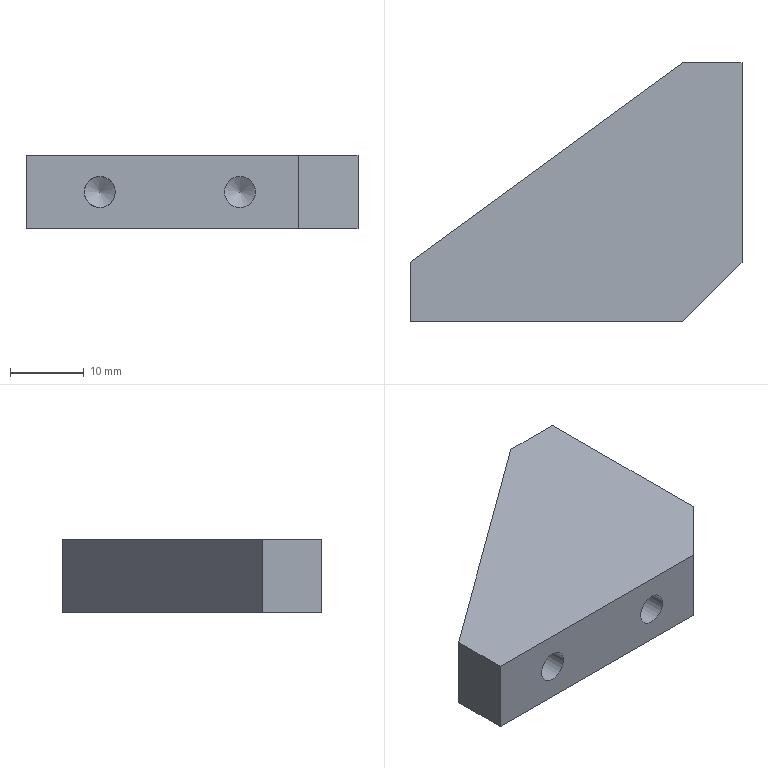Part | NX | features BREP 1 | 1 solid | 14 faces | box 45 x 35 x 10 mm | volume 9902 mm3 | plane 8 | cylinder 3 | cone 3 | commonest cylinder face diameters 4.2 x3
STEP:
#1=CARTESIAN_POINT('',(-45.,8.,10.));
#2=VERTEX_POINT('',#1);
#3=CARTESIAN_POINT('',(-45.,0.,10.));
#4=VERTEX_POINT('',#3);
#5=CARTESIAN_POINT('',(-45.,0.,10.));
#6=DIRECTION('',(0.,-1.,0.));
#7=VECTOR('',#6,1000.);
#8=LINE('',#5,#7);
#9=EDGE_CURVE('',#2,#4,#8,.T.);
#10=ORIENTED_EDGE('',*,*,#9,.T.);
#11=CARTESIAN_POINT('',(-8.,0.,10.));
#12=VERTEX_POINT('',#11);
#13=CARTESIAN_POINT('',(0.,0.,10.));
#14=DIRECTION('',(1.,0.,0.));
#15=VECTOR('',#14,1000.);
#16=LINE('',#13,#15);
#17=EDGE_CURVE('',#4,#12,#16,.T.);
#18=ORIENTED_EDGE('',*,*,#17,.T.);
#19=CARTESIAN_POINT('',(0.,8.,10.));
#20=VERTEX_POINT('',#19);
#21=CARTESIAN_POINT('',(-8.,0.,10.));
#22=DIRECTION('',(0.7071,0.7071,0.));
#23=VECTOR('',#22,1000.);
#24=LINE('',#21,#23);
#25=EDGE_CURVE('',#12,#20,#24,.T.);
#26=ORIENTED_EDGE('',*,*,#25,.T.);
#27=CARTESIAN_POINT('',(0.,35.,10.));
#28=VERTEX_POINT('',#27);
#29=CARTESIAN_POINT('',(0.,0.,10.));
#30=DIRECTION('',(0.,1.,0.));
#31=VECTOR('',#30,1000.);
#32=LINE('',#29,#31);
#33=EDGE_CURVE('',#20,#28,#32,.T.);
#34=ORIENTED_EDGE('',*,*,#33,.T.);
#35=CARTESIAN_POINT('',(-8.,35.,10.));
#36=VERTEX_POINT('',#35);
#37=CARTESIAN_POINT('',(0.,35.,10.));
#38=DIRECTION('',(-1.,0.,0.));
#39=VECTOR('',#38,1000.);
#40=LINE('',#37,#39);
#41=EDGE_CURVE('',#28,#36,#40,.T.);
#42=ORIENTED_EDGE('',*,*,#41,.T.);
#43=CARTESIAN_POINT('',(-8.,35.,10.));
#44=DIRECTION('',(-0.8078,-0.5895,0.));
#45=VECTOR('',#44,1000.);
#46=LINE('',#43,#45);
#47=EDGE_CURVE('',#36,#2,#46,.T.);
#48=ORIENTED_EDGE('',*,*,#47,.T.);
#49=EDGE_LOOP('',(#10,#18,#26,#34,#42,#48));
#50=FACE_BOUND('',#49,.T.);
#51=CARTESIAN_POINT('',(0.,0.,10.));
#52=DIRECTION('',(0.,0.,1.));
#53=DIRECTION('',(-1.,0.,0.));
#54=AXIS2_PLACEMENT_3D('',#51,#52,#53);
#55=PLANE('',#54);
#56=ADVANCED_FACE('',(#50),#55,.T.);
#57=CARTESIAN_POINT('',(-8.,0.,0.));
#58=VERTEX_POINT('',#57);
#59=CARTESIAN_POINT('',(-8.,0.,10.));
#60=DIRECTION('',(0.,0.,-1.));
#61=VECTOR('',#60,1000.);
#62=LINE('',#59,#61);
#63=EDGE_CURVE('',#12,#58,#62,.T.);
#64=ORIENTED_EDGE('',*,*,#63,.F.);
#65=ORIENTED_EDGE('',*,*,#17,.F.);
#66=CARTESIAN_POINT('',(-45.,0.,0.));
#67=VERTEX_POINT('',#66);
#68=CARTESIAN_POINT('',(-45.,0.,10.));
#69=DIRECTION('',(0.,0.,1.));
#70=VECTOR('',#69,1000.);
#71=LINE('',#68,#70);
#72=EDGE_CURVE('',#67,#4,#71,.T.);
#73=ORIENTED_EDGE('',*,*,#72,.F.);
#74=CARTESIAN_POINT('',(-45.,0.,0.));
#75=DIRECTION('',(-1.,0.,0.));
#76=VECTOR('',#75,1000.);
#77=LINE('',#74,#76);
#78=EDGE_CURVE('',#58,#67,#77,.T.);
#79=ORIENTED_EDGE('',*,*,#78,.F.);
#80=EDGE_LOOP('',(#64,#65,#73,#79));
#81=FACE_BOUND('',#80,.T.);
#82=CARTESIAN_POINT('',(-16.,0.,2.9));
#83=VERTEX_POINT('',#82);
#84=CARTESIAN_POINT('',(-16.,0.,5.));
#85=DIRECTION('',(0.,-1.,0.));
#86=DIRECTION('',(0.,0.,-1.));
#87=AXIS2_PLACEMENT_3D('',#84,#85,#86);
#88=CIRCLE('',#87,2.1);
#89=EDGE_CURVE('',#83,#83,#88,.T.);
#90=ORIENTED_EDGE('',*,*,#89,.F.);
#91=EDGE_LOOP('',(#90));
#92=FACE_BOUND('',#91,.T.);
#93=CARTESIAN_POINT('',(-35.,0.,2.9));
#94=VERTEX_POINT('',#93);
#95=CARTESIAN_POINT('',(-35.,0.,5.));
#96=DIRECTION('',(0.,-1.,0.));
#97=DIRECTION('',(0.,0.,-1.));
#98=AXIS2_PLACEMENT_3D('',#95,#96,#97);
#99=CIRCLE('',#98,2.1);
#100=EDGE_CURVE('',#94,#94,#99,.T.);
#101=ORIENTED_EDGE('',*,*,#100,.F.);
#102=EDGE_LOOP('',(#101));
#103=FACE_BOUND('',#102,.T.);
#104=CARTESIAN_POINT('',(-45.,0.,10.));
#105=DIRECTION('',(0.,1.,0.));
#106=DIRECTION('',(0.,0.,-1.));
#107=AXIS2_PLACEMENT_3D('',#104,#105,#106);
#108=PLANE('',#107);
#109=ADVANCED_FACE('',(#81,#92,#103),#108,.F.);
#110=ORIENTED_EDGE('',*,*,#72,.T.);
#111=ORIENTED_EDGE('',*,*,#9,.F.);
#112=CARTESIAN_POINT('',(-45.,8.,0.));
#113=VERTEX_POINT('',#112);
#114=CARTESIAN_POINT('',(-45.,8.,10.));
#115=DIRECTION('',(0.,0.,1.));
#116=VECTOR('',#115,1000.);
#117=LINE('',#114,#116);
#118=EDGE_CURVE('',#113,#2,#117,.T.);
#119=ORIENTED_EDGE('',*,*,#118,.F.);
#120=CARTESIAN_POINT('',(-45.,8.,0.));
#121=DIRECTION('',(0.,1.,0.));
#122=VECTOR('',#121,1000.);
#123=LINE('',#120,#122);
#124=EDGE_CURVE('',#67,#113,#123,.T.);
#125=ORIENTED_EDGE('',*,*,#124,.F.);
#126=EDGE_LOOP('',(#110,#111,#119,#125));
#127=FACE_BOUND('',#126,.T.);
#128=CARTESIAN_POINT('',(-45.,8.,10.));
#129=DIRECTION('',(1.,0.,0.));
#130=DIRECTION('',(0.,0.,1.));
#131=AXIS2_PLACEMENT_3D('',#128,#129,#130);
#132=PLANE('',#131);
#133=ADVANCED_FACE('',(#127),#132,.F.);
#134=ORIENTED_EDGE('',*,*,#118,.T.);
#135=ORIENTED_EDGE('',*,*,#47,.F.);
#136=CARTESIAN_POINT('',(-8.,35.,0.));
#137=VERTEX_POINT('',#136);
#138=CARTESIAN_POINT('',(-8.,35.,10.));
#139=DIRECTION('',(0.,0.,1.));
#140=VECTOR('',#139,1000.);
#141=LINE('',#138,#140);
#142=EDGE_CURVE('',#137,#36,#141,.T.);
#143=ORIENTED_EDGE('',*,*,#142,.F.);
#144=CARTESIAN_POINT('',(-8.,35.,0.));
#145=DIRECTION('',(0.8078,0.5895,0.));
#146=VECTOR('',#145,1000.);
#147=LINE('',#144,#146);
#148=EDGE_CURVE('',#113,#137,#147,.T.);
#149=ORIENTED_EDGE('',*,*,#148,.F.);
#150=EDGE_LOOP('',(#134,#135,#143,#149));
#151=FACE_BOUND('',#150,.T.);
#152=CARTESIAN_POINT('',(-8.,35.,10.));
#153=DIRECTION('',(0.5895,-0.8078,0.));
#154=DIRECTION('',(-0.8078,-0.5895,0.));
#155=AXIS2_PLACEMENT_3D('',#152,#153,#154);
#156=PLANE('',#155);
#157=ADVANCED_FACE('',(#151),#156,.F.);
#158=ORIENTED_EDGE('',*,*,#142,.T.);
#159=ORIENTED_EDGE('',*,*,#41,.F.);
#160=CARTESIAN_POINT('',(0.,35.,0.));
#161=VERTEX_POINT('',#160);
#162=CARTESIAN_POINT('',(0.,35.,10.));
#163=DIRECTION('',(0.,0.,1.));
#164=VECTOR('',#163,1000.);
#165=LINE('',#162,#164);
#166=EDGE_CURVE('',#161,#28,#165,.T.);
#167=ORIENTED_EDGE('',*,*,#166,.F.);
#168=CARTESIAN_POINT('',(0.,35.,0.));
#169=DIRECTION('',(1.,0.,0.));
#170=VECTOR('',#169,1000.);
#171=LINE('',#168,#170);
#172=EDGE_CURVE('',#137,#161,#171,.T.);
#173=ORIENTED_EDGE('',*,*,#172,.F.);
#174=EDGE_LOOP('',(#158,#159,#167,#173));
#175=FACE_BOUND('',#174,.T.);
#176=CARTESIAN_POINT('',(0.,35.,10.));
#177=DIRECTION('',(0.,-1.,0.));
#178=DIRECTION('',(0.,0.,1.));
#179=AXIS2_PLACEMENT_3D('',#176,#177,#178);
#180=PLANE('',#179);
#181=ADVANCED_FACE('',(#175),#180,.F.);
#182=ORIENTED_EDGE('',*,*,#166,.T.);
#183=ORIENTED_EDGE('',*,*,#33,.F.);
#184=CARTESIAN_POINT('',(0.,8.,0.));
#185=VERTEX_POINT('',#184);
#186=CARTESIAN_POINT('',(0.,8.,10.));
#187=DIRECTION('',(0.,0.,1.));
#188=VECTOR('',#187,1000.);
#189=LINE('',#186,#188);
#190=EDGE_CURVE('',#185,#20,#189,.T.);
#191=ORIENTED_EDGE('',*,*,#190,.F.);
#192=CARTESIAN_POINT('',(0.,8.,0.));
#193=DIRECTION('',(0.,-1.,0.));
#194=VECTOR('',#193,1000.);
#195=LINE('',#192,#194);
#196=EDGE_CURVE('',#161,#185,#195,.T.);
#197=ORIENTED_EDGE('',*,*,#196,.F.);
#198=EDGE_LOOP('',(#182,#183,#191,#197));
#199=FACE_BOUND('',#198,.T.);
#200=CARTESIAN_POINT('',(0.,25.,2.9));
#201=VERTEX_POINT('',#200);
#202=CARTESIAN_POINT('',(0.,25.,5.));
#203=DIRECTION('',(1.,0.,0.));
#204=DIRECTION('',(0.,0.,-1.));
#205=AXIS2_PLACEMENT_3D('',#202,#203,#204);
#206=CIRCLE('',#205,2.1);
#207=EDGE_CURVE('',#201,#201,#206,.T.);
#208=ORIENTED_EDGE('',*,*,#207,.F.);
#209=EDGE_LOOP('',(#208));
#210=FACE_BOUND('',#209,.T.);
#211=CARTESIAN_POINT('',(0.,8.,10.));
#212=DIRECTION('',(-1.,0.,0.));
#213=DIRECTION('',(0.,0.,-1.));
#214=AXIS2_PLACEMENT_3D('',#211,#212,#213);
#215=PLANE('',#214);
#216=ADVANCED_FACE('',(#199,#210),#215,.F.);
#217=ORIENTED_EDGE('',*,*,#190,.T.);
#218=ORIENTED_EDGE('',*,*,#25,.F.);
#219=ORIENTED_EDGE('',*,*,#63,.T.);
#220=CARTESIAN_POINT('',(-8.,0.,0.));
#221=DIRECTION('',(-0.7071,-0.7071,0.));
#222=VECTOR('',#221,1000.);
#223=LINE('',#220,#222);
#224=EDGE_CURVE('',#185,#58,#223,.T.);
#225=ORIENTED_EDGE('',*,*,#224,.F.);
#226=EDGE_LOOP('',(#217,#218,#219,#225));
#227=FACE_BOUND('',#226,.T.);
#228=CARTESIAN_POINT('',(-8.,0.,10.));
#229=DIRECTION('',(-0.7071,0.7071,0.));
#230=DIRECTION('',(0.7071,0.7071,0.));
#231=AXIS2_PLACEMENT_3D('',#228,#229,#230);
#232=PLANE('',#231);
#233=ADVANCED_FACE('',(#227),#232,.F.);
#234=ORIENTED_EDGE('',*,*,#78,.T.);
#235=ORIENTED_EDGE('',*,*,#124,.T.);
#236=ORIENTED_EDGE('',*,*,#148,.T.);
#237=ORIENTED_EDGE('',*,*,#172,.T.);
#238=ORIENTED_EDGE('',*,*,#196,.T.);
#239=ORIENTED_EDGE('',*,*,#224,.T.);
#240=EDGE_LOOP('',(#234,#235,#236,#237,#238,#239));
#241=FACE_BOUND('',#240,.T.);
#242=CARTESIAN_POINT('',(0.,0.,0.));
#243=DIRECTION('',(0.,0.,1.));
#244=DIRECTION('',(-1.,0.,0.));
#245=AXIS2_PLACEMENT_3D('',#242,#243,#244);
#246=PLANE('',#245);
#247=ADVANCED_FACE('',(#241),#246,.F.);
#248=CARTESIAN_POINT('',(-16.,12.4,2.9));
#249=VERTEX_POINT('',#248);
#250=CARTESIAN_POINT('',(-16.,12.4,5.));
#251=DIRECTION('',(0.,-1.,0.));
#252=DIRECTION('',(0.,0.,-1.));
#253=AXIS2_PLACEMENT_3D('',#250,#251,#252);
#254=CIRCLE('',#253,2.1);
#255=EDGE_CURVE('',#249,#249,#254,.T.);
#256=ORIENTED_EDGE('',*,*,#255,.F.);
#257=EDGE_LOOP('',(#256));
#258=FACE_BOUND('',#257,.T.);
#259=ORIENTED_EDGE('',*,*,#89,.T.);
#260=EDGE_LOOP('',(#259));
#261=FACE_BOUND('',#260,.T.);
#262=CARTESIAN_POINT('',(-16.,0.,5.));
#263=DIRECTION('',(0.,-1.,0.));
#264=DIRECTION('',(0.,0.,1.));
#265=AXIS2_PLACEMENT_3D('',#262,#263,#264);
#266=CYLINDRICAL_SURFACE('',#265,2.1);
#267=ADVANCED_FACE('',(#258,#261),#266,.F.);
#268=CARTESIAN_POINT('',(-35.,12.4,2.9));
#269=VERTEX_POINT('',#268);
#270=CARTESIAN_POINT('',(-35.,12.4,5.));
#271=DIRECTION('',(0.,-1.,0.));
#272=DIRECTION('',(0.,0.,-1.));
#273=AXIS2_PLACEMENT_3D('',#270,#271,#272);
#274=CIRCLE('',#273,2.1);
#275=EDGE_CURVE('',#269,#269,#274,.T.);
#276=ORIENTED_EDGE('',*,*,#275,.F.);
#277=EDGE_LOOP('',(#276));
#278=FACE_BOUND('',#277,.T.);
#279=ORIENTED_EDGE('',*,*,#100,.T.);
#280=EDGE_LOOP('',(#279));
#281=FACE_BOUND('',#280,.T.);
#282=CARTESIAN_POINT('',(-35.,0.,5.));
#283=DIRECTION('',(0.,-1.,0.));
#284=DIRECTION('',(0.,0.,1.));
#285=AXIS2_PLACEMENT_3D('',#282,#283,#284);
#286=CYLINDRICAL_SURFACE('',#285,2.1);
#287=ADVANCED_FACE('',(#278,#281),#286,.F.);
#288=CARTESIAN_POINT('',(-12.4,25.,2.9));
#289=VERTEX_POINT('',#288);
#290=CARTESIAN_POINT('',(-12.4,25.,5.));
#291=DIRECTION('',(1.,0.,0.));
#292=DIRECTION('',(0.,0.,-1.));
#293=AXIS2_PLACEMENT_3D('',#290,#291,#292);
#294=CIRCLE('',#293,2.1);
#295=EDGE_CURVE('',#289,#289,#294,.T.);
#296=ORIENTED_EDGE('',*,*,#295,.F.);
#297=EDGE_LOOP('',(#296));
#298=FACE_BOUND('',#297,.T.);
#299=ORIENTED_EDGE('',*,*,#207,.T.);
#300=EDGE_LOOP('',(#299));
#301=FACE_BOUND('',#300,.T.);
#302=CARTESIAN_POINT('',(0.,25.,5.));
#303=DIRECTION('',(1.,0.,0.));
#304=DIRECTION('',(0.,0.,1.));
#305=AXIS2_PLACEMENT_3D('',#302,#303,#304);
#306=CYLINDRICAL_SURFACE('',#305,2.1);
#307=ADVANCED_FACE('',(#298,#301),#306,.F.);
#308=CARTESIAN_POINT('',(-16.,13.662,5.));
#309=VERTEX_POINT('',#308);
#310=VERTEX_LOOP('',#309);
#311=FACE_BOUND('',#310,.T.);
#312=ORIENTED_EDGE('',*,*,#255,.T.);
#313=EDGE_LOOP('',(#312));
#314=FACE_BOUND('',#313,.T.);
#315=CARTESIAN_POINT('',(-16.,12.4,5.));
#316=DIRECTION('',(0.,-1.,0.));
#317=DIRECTION('',(0.,0.,1.));
#318=AXIS2_PLACEMENT_3D('',#315,#316,#317);
#319=CONICAL_SURFACE('',#318,2.1,1.03);
#320=ADVANCED_FACE('',(#311,#314),#319,.F.);
#321=CARTESIAN_POINT('',(-35.,13.662,5.));
#322=VERTEX_POINT('',#321);
#323=VERTEX_LOOP('',#322);
#324=FACE_BOUND('',#323,.T.);
#325=ORIENTED_EDGE('',*,*,#275,.T.);
#326=EDGE_LOOP('',(#325));
#327=FACE_BOUND('',#326,.T.);
#328=CARTESIAN_POINT('',(-35.,12.4,5.));
#329=DIRECTION('',(0.,-1.,0.));
#330=DIRECTION('',(-1.,0.,0.));
#331=AXIS2_PLACEMENT_3D('',#328,#329,#330);
#332=CONICAL_SURFACE('',#331,2.1,1.03);
#333=ADVANCED_FACE('',(#324,#327),#332,.F.);
#334=CARTESIAN_POINT('',(-13.662,25.,5.));
#335=VERTEX_POINT('',#334);
#336=VERTEX_LOOP('',#335);
#337=FACE_BOUND('',#336,.T.);
#338=ORIENTED_EDGE('',*,*,#295,.T.);
#339=EDGE_LOOP('',(#338));
#340=FACE_BOUND('',#339,.T.);
#341=CARTESIAN_POINT('',(-12.4,25.,5.));
#342=DIRECTION('',(1.,0.,0.));
#343=DIRECTION('',(0.,0.,1.));
#344=AXIS2_PLACEMENT_3D('',#341,#342,#343);
#345=CONICAL_SURFACE('',#344,2.1,1.03);
#346=ADVANCED_FACE('',(#337,#340),#345,.F.);
#347=CLOSED_SHELL('',(#56,#109,#133,#157,#181,#216,#233,#247,#267,#287,#307,#320,#333,#346));
#348=MANIFOLD_SOLID_BREP('',#347);
#349=(LENGTH_UNIT()NAMED_UNIT(*)SI_UNIT(.MILLI.,.METRE.));
#350=UNCERTAINTY_MEASURE_WITH_UNIT(LENGTH_MEASURE(0.00001),#349,'','');
#351=(NAMED_UNIT(*)PLANE_ANGLE_UNIT()SI_UNIT($,.RADIAN.));
#352=(NAMED_UNIT(*)SI_UNIT($,.STERADIAN.)SOLID_ANGLE_UNIT());
#353=(GEOMETRIC_REPRESENTATION_CONTEXT(3)GLOBAL_UNCERTAINTY_ASSIGNED_CONTEXT((#350))GLOBAL_UNIT_ASSIGNED_CONTEXT((#349,#351,#352))REPRESENTATION_CONTEXT('',''));
#354=ADVANCED_BREP_SHAPE_REPRESENTATION('',(#348),#353);